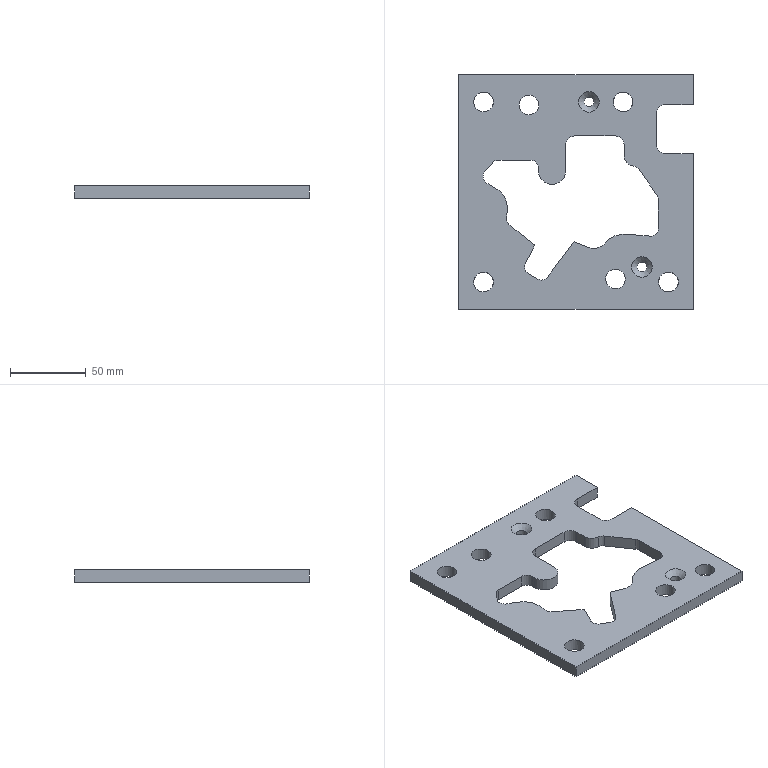Part | STEP file | gslz 2016.10.28-13_id134_x_t | 1 solid | 57 faces | box 155 x 155 x 8 mm | volume 130065 mm3 | plane 28 | cylinder 27 | cone 2 | commonest cylinder face diameters 10 x8 13 x6 12 x4 6.5 x2 14 x2 18 x2